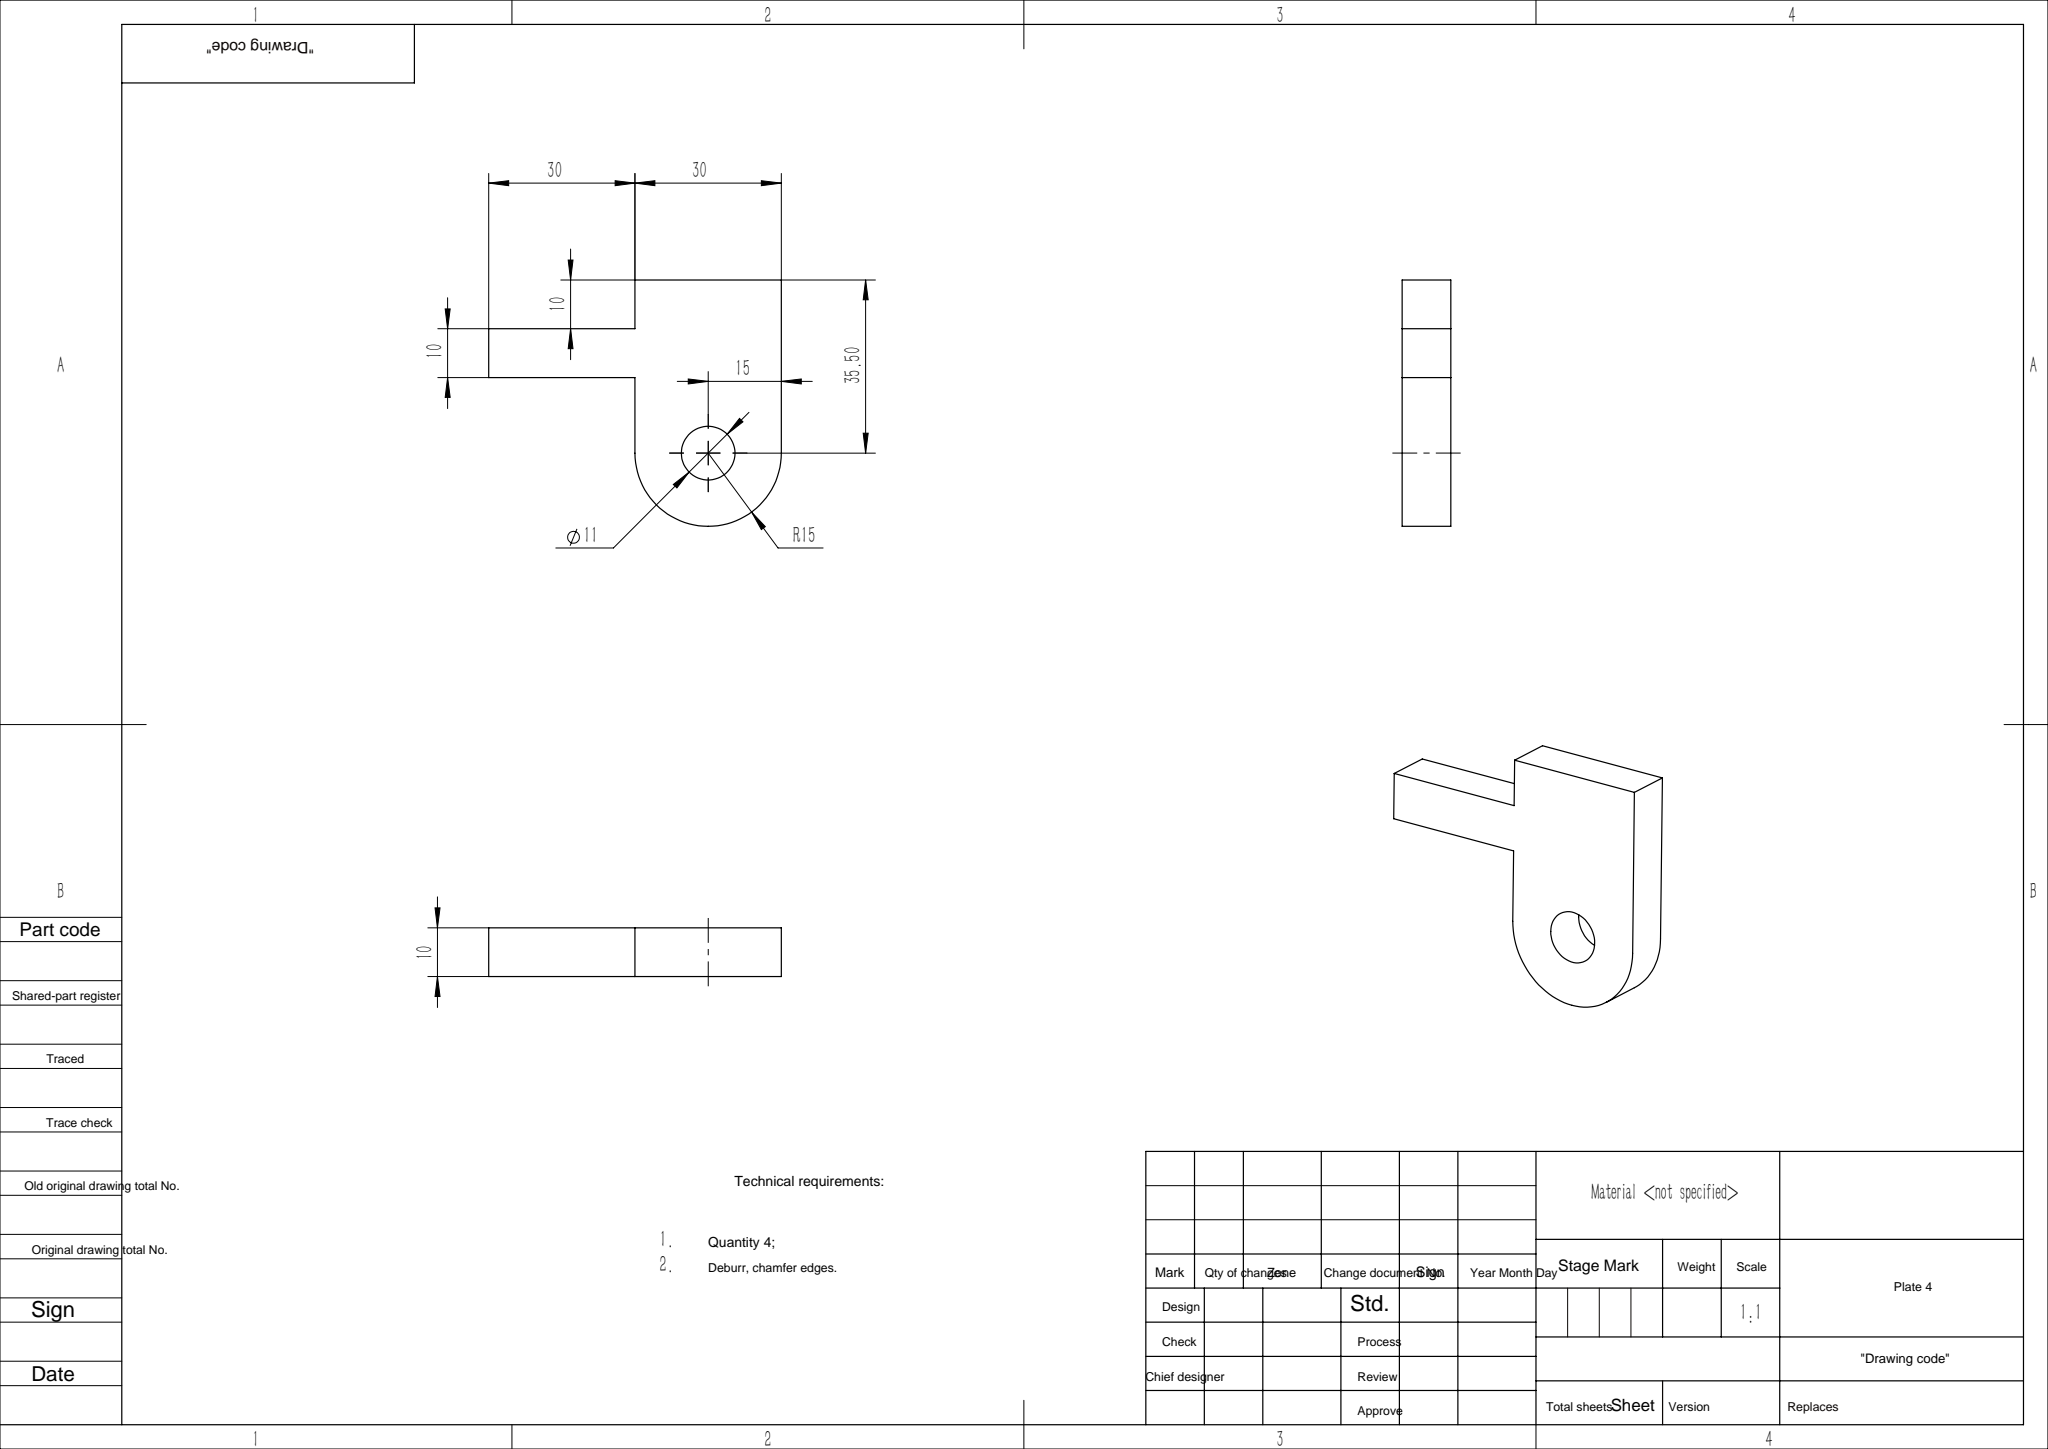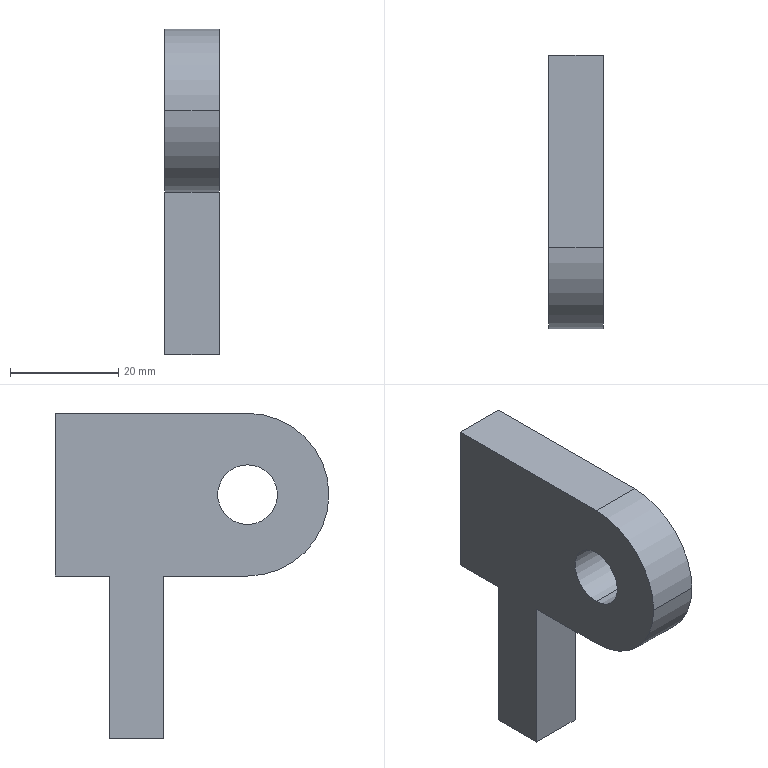Part | SolidWorks | features Extrusion 1, Fillet 1 | 1 solid | 13 faces | box 10 x 50.5 x 60 mm | volume 16234 mm3 | plane 9 | cylinder 4 | commonest cylinder face diameters 11 x2 30 x2
STEP:
#1=CARTESIAN_POINT('',(10.,-25.5,20.5));
#2=VERTEX_POINT('',#1);
#3=CARTESIAN_POINT('',(10.,-25.5,9.5));
#4=VERTEX_POINT('',#3);
#5=CARTESIAN_POINT('',(10.,-25.5,15.));
#6=DIRECTION('',(1.,0.,0.));
#7=DIRECTION('',(0.,0.,-1.));
#8=AXIS2_PLACEMENT_3D('',#5,#6,#7);
#9=CIRCLE('',#8,5.5);
#10=EDGE_CURVE('',#2,#4,#9,.T.);
#11=ORIENTED_EDGE('',*,*,#10,.T.);
#12=CARTESIAN_POINT('',(0.,-25.5,9.5));
#13=VERTEX_POINT('',#12);
#14=CARTESIAN_POINT('',(10.,-25.5,9.5));
#15=DIRECTION('',(-1.,0.,0.));
#16=VECTOR('',#15,1000.);
#17=LINE('',#14,#16);
#18=EDGE_CURVE('',#4,#13,#17,.T.);
#19=ORIENTED_EDGE('',*,*,#18,.T.);
#20=CARTESIAN_POINT('',(0.,-25.5,20.5));
#21=VERTEX_POINT('',#20);
#22=CARTESIAN_POINT('',(0.,-25.5,15.));
#23=DIRECTION('',(1.,0.,0.));
#24=DIRECTION('',(0.,0.,-1.));
#25=AXIS2_PLACEMENT_3D('',#22,#23,#24);
#26=CIRCLE('',#25,5.5);
#27=EDGE_CURVE('',#21,#13,#26,.T.);
#28=ORIENTED_EDGE('',*,*,#27,.F.);
#29=CARTESIAN_POINT('',(10.,-25.5,20.5));
#30=DIRECTION('',(-1.,0.,0.));
#31=VECTOR('',#30,1000.);
#32=LINE('',#29,#31);
#33=EDGE_CURVE('',#2,#21,#32,.T.);
#34=ORIENTED_EDGE('',*,*,#33,.F.);
#35=EDGE_LOOP('',(#11,#19,#28,#34));
#36=FACE_OUTER_BOUND('',#35,.T.);
#37=CARTESIAN_POINT('',(10.,-25.5,15.));
#38=DIRECTION('',(-1.,0.,0.));
#39=DIRECTION('',(0.,0.,1.));
#40=AXIS2_PLACEMENT_3D('',#37,#38,#39);
#41=CYLINDRICAL_SURFACE('',#40,5.5);
#42=ADVANCED_FACE('',(#36),#41,.F.);
#43=CARTESIAN_POINT('',(10.,10.,30.));
#44=VERTEX_POINT('',#43);
#45=CARTESIAN_POINT('',(10.,-25.5,30.));
#46=VERTEX_POINT('',#45);
#47=CARTESIAN_POINT('',(10.,10.,30.));
#48=DIRECTION('',(0.,-1.,0.));
#49=VECTOR('',#48,1000.);
#50=LINE('',#47,#49);
#51=EDGE_CURVE('',#44,#46,#50,.T.);
#52=ORIENTED_EDGE('',*,*,#51,.T.);
#53=CARTESIAN_POINT('',(10.,-40.5,15.));
#54=VERTEX_POINT('',#53);
#55=CARTESIAN_POINT('',(10.,-25.5,15.));
#56=DIRECTION('',(1.,0.,0.));
#57=DIRECTION('',(0.,0.,-1.));
#58=AXIS2_PLACEMENT_3D('',#55,#56,#57);
#59=CIRCLE('',#58,15.);
#60=EDGE_CURVE('',#46,#54,#59,.T.);
#61=ORIENTED_EDGE('',*,*,#60,.T.);
#62=CARTESIAN_POINT('',(10.,-25.5,0.));
#63=VERTEX_POINT('',#62);
#64=CARTESIAN_POINT('',(10.,-25.5,15.));
#65=DIRECTION('',(1.,0.,0.));
#66=DIRECTION('',(0.,0.,-1.));
#67=AXIS2_PLACEMENT_3D('',#64,#65,#66);
#68=CIRCLE('',#67,15.);
#69=EDGE_CURVE('',#54,#63,#68,.T.);
#70=ORIENTED_EDGE('',*,*,#69,.T.);
#71=CARTESIAN_POINT('',(10.,-10.,0.));
#72=VERTEX_POINT('',#71);
#73=CARTESIAN_POINT('',(10.,-10.,0.));
#74=DIRECTION('',(0.,1.,0.));
#75=VECTOR('',#74,1000.);
#76=LINE('',#73,#75);
#77=EDGE_CURVE('',#63,#72,#76,.T.);
#78=ORIENTED_EDGE('',*,*,#77,.T.);
#79=CARTESIAN_POINT('',(10.,-10.,-30.));
#80=VERTEX_POINT('',#79);
#81=CARTESIAN_POINT('',(10.,-10.,-30.));
#82=DIRECTION('',(0.,0.,-1.));
#83=VECTOR('',#82,1000.);
#84=LINE('',#81,#83);
#85=EDGE_CURVE('',#72,#80,#84,.T.);
#86=ORIENTED_EDGE('',*,*,#85,.T.);
#87=CARTESIAN_POINT('',(10.,0.,-30.));
#88=VERTEX_POINT('',#87);
#89=CARTESIAN_POINT('',(10.,0.,-30.));
#90=DIRECTION('',(0.,1.,0.));
#91=VECTOR('',#90,1000.);
#92=LINE('',#89,#91);
#93=EDGE_CURVE('',#80,#88,#92,.T.);
#94=ORIENTED_EDGE('',*,*,#93,.T.);
#95=CARTESIAN_POINT('',(10.,0.,0.));
#96=VERTEX_POINT('',#95);
#97=CARTESIAN_POINT('',(10.,0.,0.));
#98=DIRECTION('',(0.,0.,1.));
#99=VECTOR('',#98,1000.);
#100=LINE('',#97,#99);
#101=EDGE_CURVE('',#88,#96,#100,.T.);
#102=ORIENTED_EDGE('',*,*,#101,.T.);
#103=CARTESIAN_POINT('',(10.,10.,0.));
#104=VERTEX_POINT('',#103);
#105=CARTESIAN_POINT('',(10.,10.,0.));
#106=DIRECTION('',(0.,1.,0.));
#107=VECTOR('',#106,1000.);
#108=LINE('',#105,#107);
#109=EDGE_CURVE('',#96,#104,#108,.T.);
#110=ORIENTED_EDGE('',*,*,#109,.T.);
#111=CARTESIAN_POINT('',(10.,10.,0.));
#112=DIRECTION('',(0.,0.,1.));
#113=VECTOR('',#112,1000.);
#114=LINE('',#111,#113);
#115=EDGE_CURVE('',#104,#44,#114,.T.);
#116=ORIENTED_EDGE('',*,*,#115,.T.);
#117=EDGE_LOOP('',(#52,#61,#70,#78,#86,#94,#102,#110,#116));
#118=FACE_OUTER_BOUND('',#117,.T.);
#119=ORIENTED_EDGE('',*,*,#10,.F.);
#120=CARTESIAN_POINT('',(10.,-25.5,15.));
#121=DIRECTION('',(1.,0.,0.));
#122=DIRECTION('',(0.,0.,-1.));
#123=AXIS2_PLACEMENT_3D('',#120,#121,#122);
#124=CIRCLE('',#123,5.5);
#125=EDGE_CURVE('',#4,#2,#124,.T.);
#126=ORIENTED_EDGE('',*,*,#125,.F.);
#127=EDGE_LOOP('',(#119,#126));
#128=FACE_BOUND('',#127,.T.);
#129=CARTESIAN_POINT('',(10.,0.,0.));
#130=DIRECTION('',(1.,0.,0.));
#131=DIRECTION('',(0.,0.,-1.));
#132=AXIS2_PLACEMENT_3D('',#129,#130,#131);
#133=PLANE('',#132);
#134=ADVANCED_FACE('',(#118,#128),#133,.T.);
#135=CARTESIAN_POINT('',(0.,-25.5,0.));
#136=VERTEX_POINT('',#135);
#137=CARTESIAN_POINT('',(0.,-40.5,15.));
#138=VERTEX_POINT('',#137);
#139=CARTESIAN_POINT('',(0.,-25.5,15.));
#140=DIRECTION('',(-1.,0.,0.));
#141=DIRECTION('',(0.,0.,-1.));
#142=AXIS2_PLACEMENT_3D('',#139,#140,#141);
#143=CIRCLE('',#142,15.);
#144=EDGE_CURVE('',#136,#138,#143,.T.);
#145=ORIENTED_EDGE('',*,*,#144,.T.);
#146=CARTESIAN_POINT('',(0.,-25.5,30.));
#147=VERTEX_POINT('',#146);
#148=CARTESIAN_POINT('',(0.,-25.5,15.));
#149=DIRECTION('',(-1.,0.,0.));
#150=DIRECTION('',(0.,0.,-1.));
#151=AXIS2_PLACEMENT_3D('',#148,#149,#150);
#152=CIRCLE('',#151,15.);
#153=EDGE_CURVE('',#138,#147,#152,.T.);
#154=ORIENTED_EDGE('',*,*,#153,.T.);
#155=CARTESIAN_POINT('',(0.,10.,30.));
#156=VERTEX_POINT('',#155);
#157=CARTESIAN_POINT('',(0.,10.,30.));
#158=DIRECTION('',(0.,-1.,0.));
#159=VECTOR('',#158,1000.);
#160=LINE('',#157,#159);
#161=EDGE_CURVE('',#156,#147,#160,.T.);
#162=ORIENTED_EDGE('',*,*,#161,.F.);
#163=CARTESIAN_POINT('',(0.,10.,0.));
#164=VERTEX_POINT('',#163);
#165=CARTESIAN_POINT('',(0.,10.,0.));
#166=DIRECTION('',(0.,0.,1.));
#167=VECTOR('',#166,1000.);
#168=LINE('',#165,#167);
#169=EDGE_CURVE('',#164,#156,#168,.T.);
#170=ORIENTED_EDGE('',*,*,#169,.F.);
#171=CARTESIAN_POINT('',(0.,0.,0.));
#172=VERTEX_POINT('',#171);
#173=CARTESIAN_POINT('',(0.,10.,0.));
#174=DIRECTION('',(0.,1.,0.));
#175=VECTOR('',#174,1000.);
#176=LINE('',#173,#175);
#177=EDGE_CURVE('',#172,#164,#176,.T.);
#178=ORIENTED_EDGE('',*,*,#177,.F.);
#179=CARTESIAN_POINT('',(0.,0.,-30.));
#180=VERTEX_POINT('',#179);
#181=CARTESIAN_POINT('',(0.,0.,0.));
#182=DIRECTION('',(0.,0.,1.));
#183=VECTOR('',#182,1000.);
#184=LINE('',#181,#183);
#185=EDGE_CURVE('',#180,#172,#184,.T.);
#186=ORIENTED_EDGE('',*,*,#185,.F.);
#187=CARTESIAN_POINT('',(0.,-10.,-30.));
#188=VERTEX_POINT('',#187);
#189=CARTESIAN_POINT('',(0.,0.,-30.));
#190=DIRECTION('',(0.,1.,0.));
#191=VECTOR('',#190,1000.);
#192=LINE('',#189,#191);
#193=EDGE_CURVE('',#188,#180,#192,.T.);
#194=ORIENTED_EDGE('',*,*,#193,.F.);
#195=CARTESIAN_POINT('',(0.,-10.,0.));
#196=VERTEX_POINT('',#195);
#197=CARTESIAN_POINT('',(0.,-10.,-30.));
#198=DIRECTION('',(0.,0.,-1.));
#199=VECTOR('',#198,1000.);
#200=LINE('',#197,#199);
#201=EDGE_CURVE('',#196,#188,#200,.T.);
#202=ORIENTED_EDGE('',*,*,#201,.F.);
#203=CARTESIAN_POINT('',(0.,-10.,0.));
#204=DIRECTION('',(0.,1.,0.));
#205=VECTOR('',#204,1000.);
#206=LINE('',#203,#205);
#207=EDGE_CURVE('',#136,#196,#206,.T.);
#208=ORIENTED_EDGE('',*,*,#207,.F.);
#209=EDGE_LOOP('',(#145,#154,#162,#170,#178,#186,#194,#202,#208));
#210=FACE_OUTER_BOUND('',#209,.T.);
#211=ORIENTED_EDGE('',*,*,#27,.T.);
#212=CARTESIAN_POINT('',(0.,-25.5,15.));
#213=DIRECTION('',(1.,0.,0.));
#214=DIRECTION('',(0.,0.,-1.));
#215=AXIS2_PLACEMENT_3D('',#212,#213,#214);
#216=CIRCLE('',#215,5.5);
#217=EDGE_CURVE('',#13,#21,#216,.T.);
#218=ORIENTED_EDGE('',*,*,#217,.T.);
#219=EDGE_LOOP('',(#211,#218));
#220=FACE_BOUND('',#219,.T.);
#221=CARTESIAN_POINT('',(0.,0.,0.));
#222=DIRECTION('',(1.,0.,0.));
#223=DIRECTION('',(0.,0.,-1.));
#224=AXIS2_PLACEMENT_3D('',#221,#222,#223);
#225=PLANE('',#224);
#226=ADVANCED_FACE('',(#210,#220),#225,.F.);
#227=ORIENTED_EDGE('',*,*,#177,.T.);
#228=CARTESIAN_POINT('',(10.,10.,0.));
#229=DIRECTION('',(-1.,0.,0.));
#230=VECTOR('',#229,1000.);
#231=LINE('',#228,#230);
#232=EDGE_CURVE('',#104,#164,#231,.T.);
#233=ORIENTED_EDGE('',*,*,#232,.F.);
#234=ORIENTED_EDGE('',*,*,#109,.F.);
#235=CARTESIAN_POINT('',(10.,0.,0.));
#236=DIRECTION('',(-1.,0.,0.));
#237=VECTOR('',#236,1000.);
#238=LINE('',#235,#237);
#239=EDGE_CURVE('',#96,#172,#238,.T.);
#240=ORIENTED_EDGE('',*,*,#239,.T.);
#241=EDGE_LOOP('',(#227,#233,#234,#240));
#242=FACE_OUTER_BOUND('',#241,.T.);
#243=CARTESIAN_POINT('',(10.,10.,0.));
#244=DIRECTION('',(0.,0.,1.));
#245=DIRECTION('',(0.,-1.,0.));
#246=AXIS2_PLACEMENT_3D('',#243,#244,#245);
#247=PLANE('',#246);
#248=ADVANCED_FACE('',(#242),#247,.F.);
#249=ORIENTED_EDGE('',*,*,#169,.T.);
#250=CARTESIAN_POINT('',(10.,10.,30.));
#251=DIRECTION('',(-1.,0.,0.));
#252=VECTOR('',#251,1000.);
#253=LINE('',#250,#252);
#254=EDGE_CURVE('',#44,#156,#253,.T.);
#255=ORIENTED_EDGE('',*,*,#254,.F.);
#256=ORIENTED_EDGE('',*,*,#115,.F.);
#257=ORIENTED_EDGE('',*,*,#232,.T.);
#258=EDGE_LOOP('',(#249,#255,#256,#257));
#259=FACE_OUTER_BOUND('',#258,.T.);
#260=CARTESIAN_POINT('',(10.,10.,0.));
#261=DIRECTION('',(0.,-1.,0.));
#262=DIRECTION('',(0.,0.,-1.));
#263=AXIS2_PLACEMENT_3D('',#260,#261,#262);
#264=PLANE('',#263);
#265=ADVANCED_FACE('',(#259),#264,.F.);
#266=ORIENTED_EDGE('',*,*,#161,.T.);
#267=CARTESIAN_POINT('',(10.,-25.5,30.));
#268=DIRECTION('',(1.,0.,0.));
#269=VECTOR('',#268,1000.);
#270=LINE('',#267,#269);
#271=EDGE_CURVE('',#147,#46,#270,.T.);
#272=ORIENTED_EDGE('',*,*,#271,.T.);
#273=ORIENTED_EDGE('',*,*,#51,.F.);
#274=ORIENTED_EDGE('',*,*,#254,.T.);
#275=EDGE_LOOP('',(#266,#272,#273,#274));
#276=FACE_OUTER_BOUND('',#275,.T.);
#277=CARTESIAN_POINT('',(10.,10.,30.));
#278=DIRECTION('',(0.,0.,-1.));
#279=DIRECTION('',(-1.,0.,0.));
#280=AXIS2_PLACEMENT_3D('',#277,#278,#279);
#281=PLANE('',#280);
#282=ADVANCED_FACE('',(#276),#281,.F.);
#283=ORIENTED_EDGE('',*,*,#77,.F.);
#284=CARTESIAN_POINT('',(10.,-25.5,0.));
#285=DIRECTION('',(-1.,0.,0.));
#286=VECTOR('',#285,1000.);
#287=LINE('',#284,#286);
#288=EDGE_CURVE('',#63,#136,#287,.T.);
#289=ORIENTED_EDGE('',*,*,#288,.T.);
#290=ORIENTED_EDGE('',*,*,#207,.T.);
#291=CARTESIAN_POINT('',(10.,-10.,0.));
#292=DIRECTION('',(-1.,0.,0.));
#293=VECTOR('',#292,1000.);
#294=LINE('',#291,#293);
#295=EDGE_CURVE('',#72,#196,#294,.T.);
#296=ORIENTED_EDGE('',*,*,#295,.F.);
#297=EDGE_LOOP('',(#283,#289,#290,#296));
#298=FACE_OUTER_BOUND('',#297,.T.);
#299=CARTESIAN_POINT('',(10.,-10.,0.));
#300=DIRECTION('',(0.,0.,1.));
#301=DIRECTION('',(0.,-1.,0.));
#302=AXIS2_PLACEMENT_3D('',#299,#300,#301);
#303=PLANE('',#302);
#304=ADVANCED_FACE('',(#298),#303,.F.);
#305=ORIENTED_EDGE('',*,*,#201,.T.);
#306=CARTESIAN_POINT('',(10.,-10.,-30.));
#307=DIRECTION('',(-1.,0.,0.));
#308=VECTOR('',#307,1000.);
#309=LINE('',#306,#308);
#310=EDGE_CURVE('',#80,#188,#309,.T.);
#311=ORIENTED_EDGE('',*,*,#310,.F.);
#312=ORIENTED_EDGE('',*,*,#85,.F.);
#313=ORIENTED_EDGE('',*,*,#295,.T.);
#314=EDGE_LOOP('',(#305,#311,#312,#313));
#315=FACE_OUTER_BOUND('',#314,.T.);
#316=CARTESIAN_POINT('',(10.,-10.,-30.));
#317=DIRECTION('',(0.,1.,0.));
#318=DIRECTION('',(0.,0.,1.));
#319=AXIS2_PLACEMENT_3D('',#316,#317,#318);
#320=PLANE('',#319);
#321=ADVANCED_FACE('',(#315),#320,.F.);
#322=ORIENTED_EDGE('',*,*,#193,.T.);
#323=CARTESIAN_POINT('',(10.,0.,-30.));
#324=DIRECTION('',(-1.,0.,0.));
#325=VECTOR('',#324,1000.);
#326=LINE('',#323,#325);
#327=EDGE_CURVE('',#88,#180,#326,.T.);
#328=ORIENTED_EDGE('',*,*,#327,.F.);
#329=ORIENTED_EDGE('',*,*,#93,.F.);
#330=ORIENTED_EDGE('',*,*,#310,.T.);
#331=EDGE_LOOP('',(#322,#328,#329,#330));
#332=FACE_OUTER_BOUND('',#331,.T.);
#333=CARTESIAN_POINT('',(10.,0.,-30.));
#334=DIRECTION('',(0.,0.,1.));
#335=DIRECTION('',(0.,-1.,0.));
#336=AXIS2_PLACEMENT_3D('',#333,#334,#335);
#337=PLANE('',#336);
#338=ADVANCED_FACE('',(#332),#337,.F.);
#339=ORIENTED_EDGE('',*,*,#185,.T.);
#340=ORIENTED_EDGE('',*,*,#239,.F.);
#341=ORIENTED_EDGE('',*,*,#101,.F.);
#342=ORIENTED_EDGE('',*,*,#327,.T.);
#343=EDGE_LOOP('',(#339,#340,#341,#342));
#344=FACE_OUTER_BOUND('',#343,.T.);
#345=CARTESIAN_POINT('',(10.,0.,0.));
#346=DIRECTION('',(0.,-1.,0.));
#347=DIRECTION('',(0.,0.,-1.));
#348=AXIS2_PLACEMENT_3D('',#345,#346,#347);
#349=PLANE('',#348);
#350=ADVANCED_FACE('',(#344),#349,.F.);
#351=ORIENTED_EDGE('',*,*,#18,.F.);
#352=ORIENTED_EDGE('',*,*,#125,.T.);
#353=ORIENTED_EDGE('',*,*,#33,.T.);
#354=ORIENTED_EDGE('',*,*,#217,.F.);
#355=EDGE_LOOP('',(#351,#352,#353,#354));
#356=FACE_OUTER_BOUND('',#355,.T.);
#357=CARTESIAN_POINT('',(10.,-25.5,15.));
#358=DIRECTION('',(-1.,0.,0.));
#359=DIRECTION('',(0.,0.,1.));
#360=AXIS2_PLACEMENT_3D('',#357,#358,#359);
#361=CYLINDRICAL_SURFACE('',#360,5.5);
#362=ADVANCED_FACE('',(#356),#361,.F.);
#363=ORIENTED_EDGE('',*,*,#288,.F.);
#364=ORIENTED_EDGE('',*,*,#69,.F.);
#365=CARTESIAN_POINT('',(10.,-40.5,15.));
#366=DIRECTION('',(1.,0.,0.));
#367=VECTOR('',#366,1000.);
#368=LINE('',#365,#367);
#369=EDGE_CURVE('',#138,#54,#368,.T.);
#370=ORIENTED_EDGE('',*,*,#369,.F.);
#371=ORIENTED_EDGE('',*,*,#144,.F.);
#372=EDGE_LOOP('',(#363,#364,#370,#371));
#373=FACE_OUTER_BOUND('',#372,.T.);
#374=CARTESIAN_POINT('',(10.,-25.5,15.));
#375=DIRECTION('',(-1.,0.,0.));
#376=DIRECTION('',(0.,0.,1.));
#377=AXIS2_PLACEMENT_3D('',#374,#375,#376);
#378=CYLINDRICAL_SURFACE('',#377,15.);
#379=ADVANCED_FACE('',(#373),#378,.T.);
#380=ORIENTED_EDGE('',*,*,#60,.F.);
#381=ORIENTED_EDGE('',*,*,#271,.F.);
#382=ORIENTED_EDGE('',*,*,#153,.F.);
#383=ORIENTED_EDGE('',*,*,#369,.T.);
#384=EDGE_LOOP('',(#380,#381,#382,#383));
#385=FACE_OUTER_BOUND('',#384,.T.);
#386=CARTESIAN_POINT('',(10.,-25.5,15.));
#387=DIRECTION('',(-1.,0.,0.));
#388=DIRECTION('',(0.,0.,1.));
#389=AXIS2_PLACEMENT_3D('',#386,#387,#388);
#390=CYLINDRICAL_SURFACE('',#389,15.);
#391=ADVANCED_FACE('',(#385),#390,.T.);
#392=CLOSED_SHELL('',(#42,#134,#226,#248,#265,#282,#304,#321,#338,#350,#362,#379,#391));
#393=MANIFOLD_SOLID_BREP('',#392);
#394=CARTESIAN_POINT('',(0.,0.,0.));
#395=DIRECTION('',(0.,0.,1.));
#396=DIRECTION('',(1.,0.,0.));
#397=AXIS2_PLACEMENT_3D('',#394,#395,#396);
#398=(LENGTH_UNIT()NAMED_UNIT(*)SI_UNIT(.MILLI.,.METRE.));
#399=UNCERTAINTY_MEASURE_WITH_UNIT(LENGTH_MEASURE(0.00001),#398,'','');
#400=(NAMED_UNIT(*)PLANE_ANGLE_UNIT()SI_UNIT($,.RADIAN.));
#401=(NAMED_UNIT(*)SI_UNIT($,.STERADIAN.)SOLID_ANGLE_UNIT());
#402=(GEOMETRIC_REPRESENTATION_CONTEXT(3)GLOBAL_UNCERTAINTY_ASSIGNED_CONTEXT((#399))GLOBAL_UNIT_ASSIGNED_CONTEXT((#398,#400,#401))REPRESENTATION_CONTEXT('',''));
#403=ADVANCED_BREP_SHAPE_REPRESENTATION('',(#393,#397),#402);